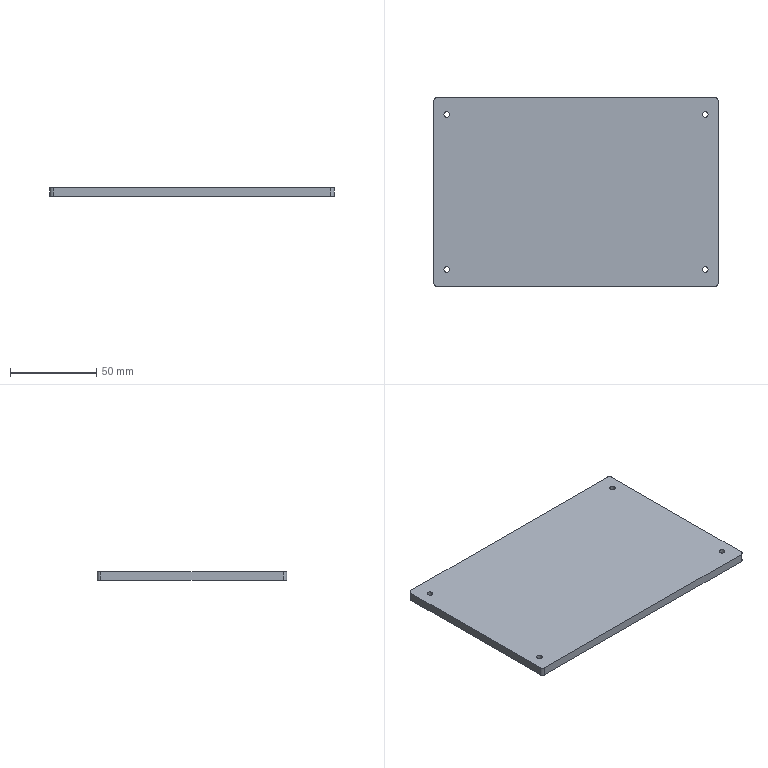Part | NX | 1 solid | 14 faces | box 165 x 110 x 5 mm | volume 90562 mm3 | cylinder 8 | plane 6 | commonest cylinder face diameters 3.3 x4 4 x4
STEP:
#1=CARTESIAN_POINT('',(82.5,-53.,5.));
#2=VERTEX_POINT('',#1);
#3=CARTESIAN_POINT('',(82.5,53.,5.));
#4=VERTEX_POINT('',#3);
#5=CARTESIAN_POINT('',(82.5,-55.,5.));
#6=DIRECTION('',(0.,1.,0.));
#7=VECTOR('',#6,1000.);
#8=LINE('',#5,#7);
#9=EDGE_CURVE('',#2,#4,#8,.T.);
#10=ORIENTED_EDGE('',*,*,#9,.F.);
#11=CARTESIAN_POINT('',(82.5,-53.,0.));
#12=VERTEX_POINT('',#11);
#13=CARTESIAN_POINT('',(82.5,-53.,5.));
#14=DIRECTION('',(0.,0.,-1.));
#15=VECTOR('',#14,1000.);
#16=LINE('',#13,#15);
#17=EDGE_CURVE('',#2,#12,#16,.T.);
#18=ORIENTED_EDGE('',*,*,#17,.T.);
#19=CARTESIAN_POINT('',(82.5,53.,0.));
#20=VERTEX_POINT('',#19);
#21=CARTESIAN_POINT('',(82.5,-55.,0.));
#22=DIRECTION('',(0.,1.,0.));
#23=VECTOR('',#22,1000.);
#24=LINE('',#21,#23);
#25=EDGE_CURVE('',#12,#20,#24,.T.);
#26=ORIENTED_EDGE('',*,*,#25,.T.);
#27=CARTESIAN_POINT('',(82.5,53.,5.));
#28=DIRECTION('',(0.,0.,-1.));
#29=VECTOR('',#28,1000.);
#30=LINE('',#27,#29);
#31=EDGE_CURVE('',#20,#4,#30,.F.);
#32=ORIENTED_EDGE('',*,*,#31,.T.);
#33=EDGE_LOOP('',(#10,#18,#26,#32));
#34=FACE_BOUND('',#33,.T.);
#35=CARTESIAN_POINT('',(82.5,-55.,5.));
#36=DIRECTION('',(-1.,0.,0.));
#37=DIRECTION('',(0.,0.,1.));
#38=AXIS2_PLACEMENT_3D('',#35,#36,#37);
#39=PLANE('',#38);
#40=ADVANCED_FACE('',(#34),#39,.F.);
#41=CARTESIAN_POINT('',(80.5,55.,5.));
#42=VERTEX_POINT('',#41);
#43=CARTESIAN_POINT('',(-80.5,55.,5.));
#44=VERTEX_POINT('',#43);
#45=CARTESIAN_POINT('',(-82.5,55.,5.));
#46=DIRECTION('',(-1.,0.,0.));
#47=VECTOR('',#46,1000.);
#48=LINE('',#45,#47);
#49=EDGE_CURVE('',#42,#44,#48,.T.);
#50=ORIENTED_EDGE('',*,*,#49,.F.);
#51=CARTESIAN_POINT('',(80.5,55.,0.));
#52=VERTEX_POINT('',#51);
#53=CARTESIAN_POINT('',(80.5,55.,5.));
#54=DIRECTION('',(0.,0.,-1.));
#55=VECTOR('',#54,1000.);
#56=LINE('',#53,#55);
#57=EDGE_CURVE('',#42,#52,#56,.T.);
#58=ORIENTED_EDGE('',*,*,#57,.T.);
#59=CARTESIAN_POINT('',(-80.5,55.,0.));
#60=VERTEX_POINT('',#59);
#61=CARTESIAN_POINT('',(-82.5,55.,0.));
#62=DIRECTION('',(-1.,0.,0.));
#63=VECTOR('',#62,1000.);
#64=LINE('',#61,#63);
#65=EDGE_CURVE('',#52,#60,#64,.T.);
#66=ORIENTED_EDGE('',*,*,#65,.T.);
#67=CARTESIAN_POINT('',(-80.5,55.,5.));
#68=DIRECTION('',(0.,0.,-1.));
#69=VECTOR('',#68,1000.);
#70=LINE('',#67,#69);
#71=EDGE_CURVE('',#60,#44,#70,.F.);
#72=ORIENTED_EDGE('',*,*,#71,.T.);
#73=EDGE_LOOP('',(#50,#58,#66,#72));
#74=FACE_BOUND('',#73,.T.);
#75=CARTESIAN_POINT('',(-82.5,55.,5.));
#76=DIRECTION('',(0.,-1.,0.));
#77=DIRECTION('',(0.,0.,-1.));
#78=AXIS2_PLACEMENT_3D('',#75,#76,#77);
#79=PLANE('',#78);
#80=ADVANCED_FACE('',(#74),#79,.F.);
#81=CARTESIAN_POINT('',(-82.5,53.,0.));
#82=VERTEX_POINT('',#81);
#83=CARTESIAN_POINT('',(-82.5,-53.,0.));
#84=VERTEX_POINT('',#83);
#85=CARTESIAN_POINT('',(-82.5,-55.,0.));
#86=DIRECTION('',(0.,-1.,0.));
#87=VECTOR('',#86,1000.);
#88=LINE('',#85,#87);
#89=EDGE_CURVE('',#82,#84,#88,.T.);
#90=ORIENTED_EDGE('',*,*,#89,.T.);
#91=CARTESIAN_POINT('',(-82.5,-53.,5.));
#92=VERTEX_POINT('',#91);
#93=CARTESIAN_POINT('',(-82.5,-53.,5.));
#94=DIRECTION('',(0.,0.,-1.));
#95=VECTOR('',#94,1000.);
#96=LINE('',#93,#95);
#97=EDGE_CURVE('',#84,#92,#96,.F.);
#98=ORIENTED_EDGE('',*,*,#97,.T.);
#99=CARTESIAN_POINT('',(-82.5,53.,5.));
#100=VERTEX_POINT('',#99);
#101=CARTESIAN_POINT('',(-82.5,-55.,5.));
#102=DIRECTION('',(0.,-1.,0.));
#103=VECTOR('',#102,1000.);
#104=LINE('',#101,#103);
#105=EDGE_CURVE('',#100,#92,#104,.T.);
#106=ORIENTED_EDGE('',*,*,#105,.F.);
#107=CARTESIAN_POINT('',(-82.5,53.,5.));
#108=DIRECTION('',(0.,0.,-1.));
#109=VECTOR('',#108,1000.);
#110=LINE('',#107,#109);
#111=EDGE_CURVE('',#100,#82,#110,.T.);
#112=ORIENTED_EDGE('',*,*,#111,.T.);
#113=EDGE_LOOP('',(#90,#98,#106,#112));
#114=FACE_BOUND('',#113,.T.);
#115=CARTESIAN_POINT('',(-82.5,-55.,5.));
#116=DIRECTION('',(1.,0.,0.));
#117=DIRECTION('',(0.,0.,-1.));
#118=AXIS2_PLACEMENT_3D('',#115,#116,#117);
#119=PLANE('',#118);
#120=ADVANCED_FACE('',(#114),#119,.F.);
#121=CARTESIAN_POINT('',(-80.5,-55.,5.));
#122=VERTEX_POINT('',#121);
#123=CARTESIAN_POINT('',(80.5,-55.,5.));
#124=VERTEX_POINT('',#123);
#125=CARTESIAN_POINT('',(-82.5,-55.,5.));
#126=DIRECTION('',(1.,0.,0.));
#127=VECTOR('',#126,1000.);
#128=LINE('',#125,#127);
#129=EDGE_CURVE('',#122,#124,#128,.T.);
#130=ORIENTED_EDGE('',*,*,#129,.F.);
#131=CARTESIAN_POINT('',(-80.5,-55.,0.));
#132=VERTEX_POINT('',#131);
#133=CARTESIAN_POINT('',(-80.5,-55.,5.));
#134=DIRECTION('',(0.,0.,-1.));
#135=VECTOR('',#134,1000.);
#136=LINE('',#133,#135);
#137=EDGE_CURVE('',#122,#132,#136,.T.);
#138=ORIENTED_EDGE('',*,*,#137,.T.);
#139=CARTESIAN_POINT('',(80.5,-55.,0.));
#140=VERTEX_POINT('',#139);
#141=CARTESIAN_POINT('',(-82.5,-55.,0.));
#142=DIRECTION('',(1.,0.,0.));
#143=VECTOR('',#142,1000.);
#144=LINE('',#141,#143);
#145=EDGE_CURVE('',#132,#140,#144,.T.);
#146=ORIENTED_EDGE('',*,*,#145,.T.);
#147=CARTESIAN_POINT('',(80.5,-55.,5.));
#148=DIRECTION('',(0.,0.,-1.));
#149=VECTOR('',#148,1000.);
#150=LINE('',#147,#149);
#151=EDGE_CURVE('',#140,#124,#150,.F.);
#152=ORIENTED_EDGE('',*,*,#151,.T.);
#153=EDGE_LOOP('',(#130,#138,#146,#152));
#154=FACE_BOUND('',#153,.T.);
#155=CARTESIAN_POINT('',(-82.5,-55.,5.));
#156=DIRECTION('',(0.,1.,0.));
#157=DIRECTION('',(0.,0.,1.));
#158=AXIS2_PLACEMENT_3D('',#155,#156,#157);
#159=PLANE('',#158);
#160=ADVANCED_FACE('',(#154),#159,.F.);
#161=CARTESIAN_POINT('',(-73.35,45.,5.));
#162=VERTEX_POINT('',#161);
#163=CARTESIAN_POINT('',(-75.,45.,5.));
#164=DIRECTION('',(0.,0.,1.));
#165=DIRECTION('',(1.,0.,0.));
#166=AXIS2_PLACEMENT_3D('',#163,#164,#165);
#167=CIRCLE('',#166,1.65);
#168=EDGE_CURVE('',#162,#162,#167,.T.);
#169=ORIENTED_EDGE('',*,*,#168,.F.);
#170=EDGE_LOOP('',(#169));
#171=FACE_BOUND('',#170,.T.);
#172=CARTESIAN_POINT('',(76.65,45.,5.));
#173=VERTEX_POINT('',#172);
#174=CARTESIAN_POINT('',(75.,45.,5.));
#175=DIRECTION('',(0.,0.,1.));
#176=DIRECTION('',(1.,0.,0.));
#177=AXIS2_PLACEMENT_3D('',#174,#175,#176);
#178=CIRCLE('',#177,1.65);
#179=EDGE_CURVE('',#173,#173,#178,.T.);
#180=ORIENTED_EDGE('',*,*,#179,.F.);
#181=EDGE_LOOP('',(#180));
#182=FACE_BOUND('',#181,.T.);
#183=CARTESIAN_POINT('',(76.65,-45.,5.));
#184=VERTEX_POINT('',#183);
#185=CARTESIAN_POINT('',(75.,-45.,5.));
#186=DIRECTION('',(0.,0.,1.));
#187=DIRECTION('',(1.,0.,0.));
#188=AXIS2_PLACEMENT_3D('',#185,#186,#187);
#189=CIRCLE('',#188,1.65);
#190=EDGE_CURVE('',#184,#184,#189,.T.);
#191=ORIENTED_EDGE('',*,*,#190,.F.);
#192=EDGE_LOOP('',(#191));
#193=FACE_BOUND('',#192,.T.);
#194=CARTESIAN_POINT('',(-73.35,-45.,5.));
#195=VERTEX_POINT('',#194);
#196=CARTESIAN_POINT('',(-75.,-45.,5.));
#197=DIRECTION('',(0.,0.,1.));
#198=DIRECTION('',(1.,0.,0.));
#199=AXIS2_PLACEMENT_3D('',#196,#197,#198);
#200=CIRCLE('',#199,1.65);
#201=EDGE_CURVE('',#195,#195,#200,.T.);
#202=ORIENTED_EDGE('',*,*,#201,.F.);
#203=EDGE_LOOP('',(#202));
#204=FACE_BOUND('',#203,.T.);
#205=ORIENTED_EDGE('',*,*,#105,.T.);
#206=CARTESIAN_POINT('',(-80.5,-53.,5.));
#207=DIRECTION('',(0.,0.,-1.));
#208=DIRECTION('',(-1.,0.,0.));
#209=AXIS2_PLACEMENT_3D('',#206,#207,#208);
#210=CIRCLE('',#209,2.);
#211=EDGE_CURVE('',#92,#122,#210,.F.);
#212=ORIENTED_EDGE('',*,*,#211,.T.);
#213=ORIENTED_EDGE('',*,*,#129,.T.);
#214=CARTESIAN_POINT('',(80.5,-53.,5.));
#215=DIRECTION('',(0.,0.,-1.));
#216=DIRECTION('',(-1.,0.,0.));
#217=AXIS2_PLACEMENT_3D('',#214,#215,#216);
#218=CIRCLE('',#217,2.);
#219=EDGE_CURVE('',#124,#2,#218,.F.);
#220=ORIENTED_EDGE('',*,*,#219,.T.);
#221=ORIENTED_EDGE('',*,*,#9,.T.);
#222=CARTESIAN_POINT('',(80.5,53.,5.));
#223=DIRECTION('',(0.,0.,-1.));
#224=DIRECTION('',(-1.,0.,0.));
#225=AXIS2_PLACEMENT_3D('',#222,#223,#224);
#226=CIRCLE('',#225,2.);
#227=EDGE_CURVE('',#4,#42,#226,.F.);
#228=ORIENTED_EDGE('',*,*,#227,.T.);
#229=ORIENTED_EDGE('',*,*,#49,.T.);
#230=CARTESIAN_POINT('',(-80.5,53.,5.));
#231=DIRECTION('',(0.,0.,-1.));
#232=DIRECTION('',(-1.,0.,0.));
#233=AXIS2_PLACEMENT_3D('',#230,#231,#232);
#234=CIRCLE('',#233,2.);
#235=EDGE_CURVE('',#44,#100,#234,.F.);
#236=ORIENTED_EDGE('',*,*,#235,.T.);
#237=EDGE_LOOP('',(#205,#212,#213,#220,#221,#228,#229,#236));
#238=FACE_BOUND('',#237,.T.);
#239=CARTESIAN_POINT('',(0.,0.,5.));
#240=DIRECTION('',(0.,0.,-1.));
#241=DIRECTION('',(-1.,0.,0.));
#242=AXIS2_PLACEMENT_3D('',#239,#240,#241);
#243=PLANE('',#242);
#244=ADVANCED_FACE('',(#171,#182,#193,#204,#238),#243,.F.);
#245=CARTESIAN_POINT('',(-73.35,45.,0.));
#246=VERTEX_POINT('',#245);
#247=CARTESIAN_POINT('',(-75.,45.,0.));
#248=DIRECTION('',(0.,0.,1.));
#249=DIRECTION('',(1.,0.,0.));
#250=AXIS2_PLACEMENT_3D('',#247,#248,#249);
#251=CIRCLE('',#250,1.65);
#252=EDGE_CURVE('',#246,#246,#251,.T.);
#253=ORIENTED_EDGE('',*,*,#252,.T.);
#254=EDGE_LOOP('',(#253));
#255=FACE_BOUND('',#254,.T.);
#256=CARTESIAN_POINT('',(76.65,45.,0.));
#257=VERTEX_POINT('',#256);
#258=CARTESIAN_POINT('',(75.,45.,0.));
#259=DIRECTION('',(0.,0.,1.));
#260=DIRECTION('',(1.,0.,0.));
#261=AXIS2_PLACEMENT_3D('',#258,#259,#260);
#262=CIRCLE('',#261,1.65);
#263=EDGE_CURVE('',#257,#257,#262,.T.);
#264=ORIENTED_EDGE('',*,*,#263,.T.);
#265=EDGE_LOOP('',(#264));
#266=FACE_BOUND('',#265,.T.);
#267=CARTESIAN_POINT('',(76.65,-45.,0.));
#268=VERTEX_POINT('',#267);
#269=CARTESIAN_POINT('',(75.,-45.,0.));
#270=DIRECTION('',(0.,0.,1.));
#271=DIRECTION('',(1.,0.,0.));
#272=AXIS2_PLACEMENT_3D('',#269,#270,#271);
#273=CIRCLE('',#272,1.65);
#274=EDGE_CURVE('',#268,#268,#273,.T.);
#275=ORIENTED_EDGE('',*,*,#274,.T.);
#276=EDGE_LOOP('',(#275));
#277=FACE_BOUND('',#276,.T.);
#278=CARTESIAN_POINT('',(-73.35,-45.,0.));
#279=VERTEX_POINT('',#278);
#280=CARTESIAN_POINT('',(-75.,-45.,0.));
#281=DIRECTION('',(0.,0.,1.));
#282=DIRECTION('',(1.,0.,0.));
#283=AXIS2_PLACEMENT_3D('',#280,#281,#282);
#284=CIRCLE('',#283,1.65);
#285=EDGE_CURVE('',#279,#279,#284,.T.);
#286=ORIENTED_EDGE('',*,*,#285,.T.);
#287=EDGE_LOOP('',(#286));
#288=FACE_BOUND('',#287,.T.);
#289=ORIENTED_EDGE('',*,*,#145,.F.);
#290=CARTESIAN_POINT('',(-80.5,-53.,0.));
#291=DIRECTION('',(0.,0.,-1.));
#292=DIRECTION('',(-1.,0.,0.));
#293=AXIS2_PLACEMENT_3D('',#290,#291,#292);
#294=CIRCLE('',#293,2.);
#295=EDGE_CURVE('',#132,#84,#294,.T.);
#296=ORIENTED_EDGE('',*,*,#295,.T.);
#297=ORIENTED_EDGE('',*,*,#89,.F.);
#298=CARTESIAN_POINT('',(-80.5,53.,0.));
#299=DIRECTION('',(0.,0.,-1.));
#300=DIRECTION('',(-1.,0.,0.));
#301=AXIS2_PLACEMENT_3D('',#298,#299,#300);
#302=CIRCLE('',#301,2.);
#303=EDGE_CURVE('',#82,#60,#302,.T.);
#304=ORIENTED_EDGE('',*,*,#303,.T.);
#305=ORIENTED_EDGE('',*,*,#65,.F.);
#306=CARTESIAN_POINT('',(80.5,53.,0.));
#307=DIRECTION('',(0.,0.,-1.));
#308=DIRECTION('',(-1.,0.,0.));
#309=AXIS2_PLACEMENT_3D('',#306,#307,#308);
#310=CIRCLE('',#309,2.);
#311=EDGE_CURVE('',#52,#20,#310,.T.);
#312=ORIENTED_EDGE('',*,*,#311,.T.);
#313=ORIENTED_EDGE('',*,*,#25,.F.);
#314=CARTESIAN_POINT('',(80.5,-53.,0.));
#315=DIRECTION('',(0.,0.,-1.));
#316=DIRECTION('',(-1.,0.,0.));
#317=AXIS2_PLACEMENT_3D('',#314,#315,#316);
#318=CIRCLE('',#317,2.);
#319=EDGE_CURVE('',#12,#140,#318,.T.);
#320=ORIENTED_EDGE('',*,*,#319,.T.);
#321=EDGE_LOOP('',(#289,#296,#297,#304,#305,#312,#313,#320));
#322=FACE_BOUND('',#321,.T.);
#323=CARTESIAN_POINT('',(0.,0.,0.));
#324=DIRECTION('',(0.,0.,-1.));
#325=DIRECTION('',(-1.,0.,0.));
#326=AXIS2_PLACEMENT_3D('',#323,#324,#325);
#327=PLANE('',#326);
#328=ADVANCED_FACE('',(#255,#266,#277,#288,#322),#327,.T.);
#329=ORIENTED_EDGE('',*,*,#285,.F.);
#330=EDGE_LOOP('',(#329));
#331=FACE_BOUND('',#330,.T.);
#332=ORIENTED_EDGE('',*,*,#201,.T.);
#333=EDGE_LOOP('',(#332));
#334=FACE_BOUND('',#333,.T.);
#335=CARTESIAN_POINT('',(-75.,-45.,5.));
#336=DIRECTION('',(0.,0.,1.));
#337=DIRECTION('',(1.,0.,0.));
#338=AXIS2_PLACEMENT_3D('',#335,#336,#337);
#339=CYLINDRICAL_SURFACE('',#338,1.65);
#340=ADVANCED_FACE('',(#331,#334),#339,.F.);
#341=ORIENTED_EDGE('',*,*,#274,.F.);
#342=EDGE_LOOP('',(#341));
#343=FACE_BOUND('',#342,.T.);
#344=ORIENTED_EDGE('',*,*,#190,.T.);
#345=EDGE_LOOP('',(#344));
#346=FACE_BOUND('',#345,.T.);
#347=CARTESIAN_POINT('',(75.,-45.,5.));
#348=DIRECTION('',(0.,0.,1.));
#349=DIRECTION('',(1.,0.,0.));
#350=AXIS2_PLACEMENT_3D('',#347,#348,#349);
#351=CYLINDRICAL_SURFACE('',#350,1.65);
#352=ADVANCED_FACE('',(#343,#346),#351,.F.);
#353=ORIENTED_EDGE('',*,*,#263,.F.);
#354=EDGE_LOOP('',(#353));
#355=FACE_BOUND('',#354,.T.);
#356=ORIENTED_EDGE('',*,*,#179,.T.);
#357=EDGE_LOOP('',(#356));
#358=FACE_BOUND('',#357,.T.);
#359=CARTESIAN_POINT('',(75.,45.,5.));
#360=DIRECTION('',(0.,0.,1.));
#361=DIRECTION('',(1.,0.,0.));
#362=AXIS2_PLACEMENT_3D('',#359,#360,#361);
#363=CYLINDRICAL_SURFACE('',#362,1.65);
#364=ADVANCED_FACE('',(#355,#358),#363,.F.);
#365=ORIENTED_EDGE('',*,*,#252,.F.);
#366=EDGE_LOOP('',(#365));
#367=FACE_BOUND('',#366,.T.);
#368=ORIENTED_EDGE('',*,*,#168,.T.);
#369=EDGE_LOOP('',(#368));
#370=FACE_BOUND('',#369,.T.);
#371=CARTESIAN_POINT('',(-75.,45.,5.));
#372=DIRECTION('',(0.,0.,1.));
#373=DIRECTION('',(1.,0.,0.));
#374=AXIS2_PLACEMENT_3D('',#371,#372,#373);
#375=CYLINDRICAL_SURFACE('',#374,1.65);
#376=ADVANCED_FACE('',(#367,#370),#375,.F.);
#377=ORIENTED_EDGE('',*,*,#211,.F.);
#378=ORIENTED_EDGE('',*,*,#97,.F.);
#379=ORIENTED_EDGE('',*,*,#295,.F.);
#380=ORIENTED_EDGE('',*,*,#137,.F.);
#381=EDGE_LOOP('',(#377,#378,#379,#380));
#382=FACE_BOUND('',#381,.T.);
#383=CARTESIAN_POINT('',(-80.5,-53.,5.));
#384=DIRECTION('',(0.,0.,-1.));
#385=DIRECTION('',(-1.,0.,0.));
#386=AXIS2_PLACEMENT_3D('',#383,#384,#385);
#387=CYLINDRICAL_SURFACE('',#386,2.);
#388=ADVANCED_FACE('',(#382),#387,.T.);
#389=ORIENTED_EDGE('',*,*,#219,.F.);
#390=ORIENTED_EDGE('',*,*,#151,.F.);
#391=ORIENTED_EDGE('',*,*,#319,.F.);
#392=ORIENTED_EDGE('',*,*,#17,.F.);
#393=EDGE_LOOP('',(#389,#390,#391,#392));
#394=FACE_BOUND('',#393,.T.);
#395=CARTESIAN_POINT('',(80.5,-53.,5.));
#396=DIRECTION('',(0.,0.,-1.));
#397=DIRECTION('',(-1.,0.,0.));
#398=AXIS2_PLACEMENT_3D('',#395,#396,#397);
#399=CYLINDRICAL_SURFACE('',#398,2.);
#400=ADVANCED_FACE('',(#394),#399,.T.);
#401=ORIENTED_EDGE('',*,*,#227,.F.);
#402=ORIENTED_EDGE('',*,*,#31,.F.);
#403=ORIENTED_EDGE('',*,*,#311,.F.);
#404=ORIENTED_EDGE('',*,*,#57,.F.);
#405=EDGE_LOOP('',(#401,#402,#403,#404));
#406=FACE_BOUND('',#405,.T.);
#407=CARTESIAN_POINT('',(80.5,53.,5.));
#408=DIRECTION('',(0.,0.,-1.));
#409=DIRECTION('',(-1.,0.,0.));
#410=AXIS2_PLACEMENT_3D('',#407,#408,#409);
#411=CYLINDRICAL_SURFACE('',#410,2.);
#412=ADVANCED_FACE('',(#406),#411,.T.);
#413=ORIENTED_EDGE('',*,*,#235,.F.);
#414=ORIENTED_EDGE('',*,*,#71,.F.);
#415=ORIENTED_EDGE('',*,*,#303,.F.);
#416=ORIENTED_EDGE('',*,*,#111,.F.);
#417=EDGE_LOOP('',(#413,#414,#415,#416));
#418=FACE_BOUND('',#417,.T.);
#419=CARTESIAN_POINT('',(-80.5,53.,5.));
#420=DIRECTION('',(0.,0.,-1.));
#421=DIRECTION('',(-1.,0.,0.));
#422=AXIS2_PLACEMENT_3D('',#419,#420,#421);
#423=CYLINDRICAL_SURFACE('',#422,2.);
#424=ADVANCED_FACE('',(#418),#423,.T.);
#425=CLOSED_SHELL('',(#40,#80,#120,#160,#244,#328,#340,#352,#364,#376,#388,#400,#412,#424));
#426=MANIFOLD_SOLID_BREP('',#425);
#427=(LENGTH_UNIT()NAMED_UNIT(*)SI_UNIT(.MILLI.,.METRE.));
#428=UNCERTAINTY_MEASURE_WITH_UNIT(LENGTH_MEASURE(0.00001),#427,'','');
#429=(NAMED_UNIT(*)PLANE_ANGLE_UNIT()SI_UNIT($,.RADIAN.));
#430=(NAMED_UNIT(*)SI_UNIT($,.STERADIAN.)SOLID_ANGLE_UNIT());
#431=(GEOMETRIC_REPRESENTATION_CONTEXT(3)GLOBAL_UNCERTAINTY_ASSIGNED_CONTEXT((#428))GLOBAL_UNIT_ASSIGNED_CONTEXT((#427,#429,#430))REPRESENTATION_CONTEXT('',''));
#432=ADVANCED_BREP_SHAPE_REPRESENTATION('',(#426),#431);